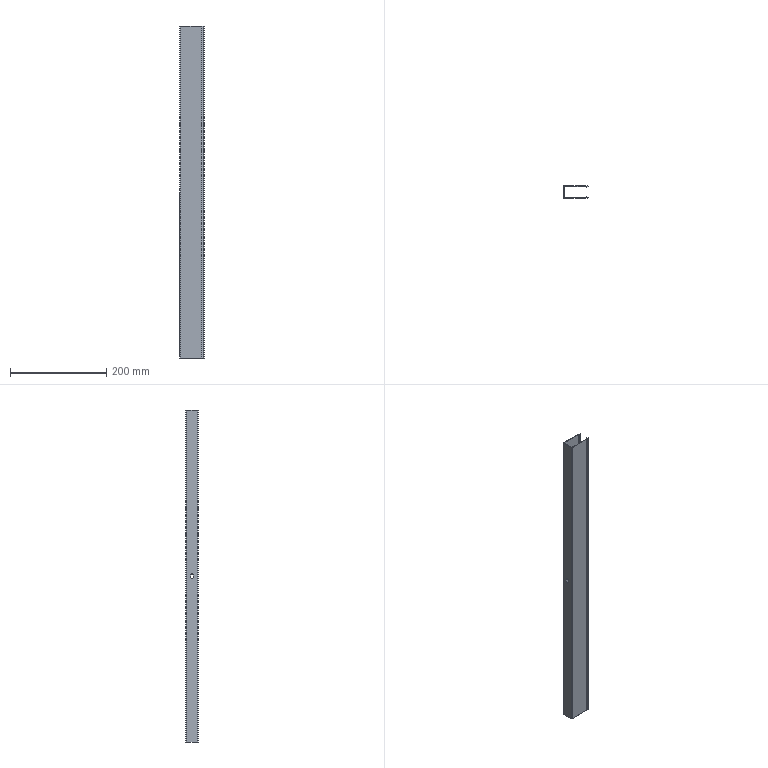Part | STEP file | Cable trough 4 | 1 solid | 27 faces | box 50.625 x 25 x 690 mm | volume 86789 mm3 | plane 20 | cylinder 7 | commonest cylinder face diameters 5 x3 1 x2 3 x2